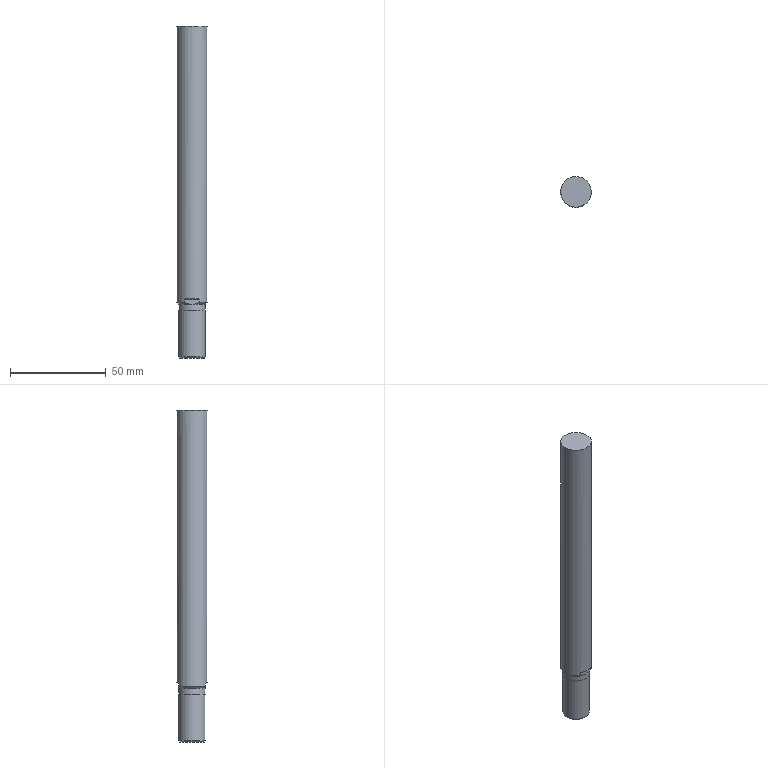Part | STEP file | 冲床-300配套压波_id650_x_t | 1 solid | 14 faces | box 16 x 16 x 173 mm | volume 33408 mm3 | plane 6 | cylinder 5 | cone 3 | commonest cylinder face diameters 1 x2 14 x2 16 x1
STEP:
#1=CARTESIAN_POINT('',(1812.,0.,183.7));
#2=VERTEX_POINT('',#1);
#3=CARTESIAN_POINT('',(1805.,0.,183.7));
#4=DIRECTION('',(0.,0.,1.));
#5=DIRECTION('',(1.,0.,0.));
#6=AXIS2_PLACEMENT_3D('',#3,#4,#5);
#7=CIRCLE('',#6,7.);
#8=EDGE_CURVE('',#2,#2,#7,.T.);
#9=ORIENTED_EDGE('',*,*,#8,.T.);
#10=EDGE_LOOP('',(#9));
#11=FACE_BOUND('',#10,.T.);
#12=CARTESIAN_POINT('',(1798.,0.,208.));
#13=VERTEX_POINT('',#12);
#14=CARTESIAN_POINT('',(1805.,0.,208.));
#15=DIRECTION('',(0.,0.,-1.));
#16=DIRECTION('',(-1.,0.,0.));
#17=AXIS2_PLACEMENT_3D('',#14,#15,#16);
#18=CIRCLE('',#17,7.);
#19=EDGE_CURVE('',#13,#13,#18,.T.);
#20=ORIENTED_EDGE('',*,*,#19,.T.);
#21=EDGE_LOOP('',(#20));
#22=FACE_BOUND('',#21,.T.);
#23=CARTESIAN_POINT('',(1805.,0.,211.));
#24=DIRECTION('',(0.,0.,-1.));
#25=DIRECTION('',(1.,0.,0.));
#26=AXIS2_PLACEMENT_3D('',#23,#24,#25);
#27=CYLINDRICAL_SURFACE('',#26,7.);
#28=ADVANCED_FACE('',(#11,#22),#27,.T.);
#29=CARTESIAN_POINT('',(1801.127,7.,213.3));
#30=VERTEX_POINT('',#29);
#31=CARTESIAN_POINT('',(1801.127,7.,212.));
#32=VERTEX_POINT('',#31);
#33=CARTESIAN_POINT('',(1801.127,7.,213.8));
#34=DIRECTION('',(0.,0.,-1.));
#35=VECTOR('',#34,1.);
#36=LINE('',#33,#35);
#37=EDGE_CURVE('',#30,#32,#36,.T.);
#38=ORIENTED_EDGE('',*,*,#37,.T.);
#39=CARTESIAN_POINT('',(1801.127,-7.,212.));
#40=VERTEX_POINT('',#39);
#41=CARTESIAN_POINT('',(1805.,0.,212.));
#42=DIRECTION('',(0.,0.,1.));
#43=DIRECTION('',(-1.,0.,0.));
#44=AXIS2_PLACEMENT_3D('',#41,#42,#43);
#45=CIRCLE('',#44,8.);
#46=EDGE_CURVE('',#32,#40,#45,.T.);
#47=ORIENTED_EDGE('',*,*,#46,.T.);
#48=CARTESIAN_POINT('',(1801.127,-7.,213.3));
#49=VERTEX_POINT('',#48);
#50=CARTESIAN_POINT('',(1801.127,-7.,213.8));
#51=DIRECTION('',(0.,0.,-1.));
#52=VECTOR('',#51,1.);
#53=LINE('',#50,#52);
#54=EDGE_CURVE('',#49,#40,#53,.T.);
#55=ORIENTED_EDGE('',*,*,#54,.F.);
#56=CARTESIAN_POINT('',(1802.216,-7.5,213.8));
#57=VERTEX_POINT('',#56);
#58=CARTESIAN_POINT('',(1801.127,-7.,213.3));
#59=CARTESIAN_POINT('',(1801.127,-7.,213.329));
#60=CARTESIAN_POINT('',(1801.132,-7.003,213.358));
#61=CARTESIAN_POINT('',(1801.14,-7.007,213.385));
#62=CARTESIAN_POINT('',(1801.151,-7.013,213.419));
#63=CARTESIAN_POINT('',(1801.167,-7.022,213.45));
#64=CARTESIAN_POINT('',(1801.186,-7.032,213.477));
#65=CARTESIAN_POINT('',(1801.216,-7.048,213.519));
#66=CARTESIAN_POINT('',(1801.253,-7.068,213.555));
#67=CARTESIAN_POINT('',(1801.292,-7.089,213.584));
#68=CARTESIAN_POINT('',(1801.365,-7.127,213.64));
#69=CARTESIAN_POINT('',(1801.449,-7.169,213.678));
#70=CARTESIAN_POINT('',(1801.534,-7.21,213.708));
#71=CARTESIAN_POINT('',(1801.718,-7.298,213.77));
#72=CARTESIAN_POINT('',(1801.916,-7.385,213.793));
#73=CARTESIAN_POINT('',(1802.115,-7.462,213.799));
#74=CARTESIAN_POINT('',(1802.148,-7.475,213.8));
#75=CARTESIAN_POINT('',(1802.182,-7.487,213.8));
#76=CARTESIAN_POINT('',(1802.216,-7.5,213.8));
#77=B_SPLINE_CURVE_WITH_KNOTS('',3,(#58,#59,#60,#61,#62,#63,#64,#65,#66,#67,#68,#69,#70,#71,#72,#73,#74,#75,#76),.UNSPECIFIED.,.F.,.F.,(4,3,3,3,3,3,4),(0.,0.06162,0.1366,0.2512,0.4638,0.9227,1.),.UNSPECIFIED.);
#78=EDGE_CURVE('',#49,#57,#77,.T.);
#79=ORIENTED_EDGE('',*,*,#78,.T.);
#80=CARTESIAN_POINT('',(1807.784,-7.5,213.8));
#81=VERTEX_POINT('',#80);
#82=CARTESIAN_POINT('',(1805.,0.,213.8));
#83=DIRECTION('',(0.,0.,-1.));
#84=DIRECTION('',(-1.,0.,0.));
#85=AXIS2_PLACEMENT_3D('',#82,#83,#84);
#86=CIRCLE('',#85,8.);
#87=EDGE_CURVE('',#81,#57,#86,.T.);
#88=ORIENTED_EDGE('',*,*,#87,.F.);
#89=CARTESIAN_POINT('',(1808.873,-7.,213.3));
#90=VERTEX_POINT('',#89);
#91=CARTESIAN_POINT('',(1807.784,-7.5,213.8));
#92=CARTESIAN_POINT('',(1807.985,-7.425,213.8));
#93=CARTESIAN_POINT('',(1808.186,-7.341,213.785));
#94=CARTESIAN_POINT('',(1808.376,-7.253,213.735));
#95=CARTESIAN_POINT('',(1808.44,-7.223,213.718));
#96=CARTESIAN_POINT('',(1808.504,-7.192,213.696));
#97=CARTESIAN_POINT('',(1808.564,-7.162,213.669));
#98=CARTESIAN_POINT('',(1808.642,-7.123,213.633));
#99=CARTESIAN_POINT('',(1808.719,-7.084,213.586));
#100=CARTESIAN_POINT('',(1808.779,-7.051,213.521));
#101=CARTESIAN_POINT('',(1808.801,-7.039,213.496));
#102=CARTESIAN_POINT('',(1808.822,-7.028,213.469));
#103=CARTESIAN_POINT('',(1808.838,-7.019,213.438));
#104=CARTESIAN_POINT('',(1808.854,-7.011,213.407));
#105=CARTESIAN_POINT('',(1808.866,-7.004,213.373));
#106=CARTESIAN_POINT('',(1808.87,-7.001,213.337));
#107=CARTESIAN_POINT('',(1808.872,-7.,213.325));
#108=CARTESIAN_POINT('',(1808.873,-7.,213.312));
#109=CARTESIAN_POINT('',(1808.873,-7.,213.3));
#110=B_SPLINE_CURVE_WITH_KNOTS('',3,(#91,#92,#93,#94,#95,#96,#97,#98,#99,#100,#101,#102,#103,#104,#105,#106,#107,#108,#109),.UNSPECIFIED.,.F.,.F.,(4,3,3,3,3,3,4),(0.,0.4621,0.6184,0.8217,0.8971,0.9738,1.),.UNSPECIFIED.);
#111=EDGE_CURVE('',#81,#90,#110,.T.);
#112=ORIENTED_EDGE('',*,*,#111,.T.);
#113=CARTESIAN_POINT('',(1808.873,-7.,212.));
#114=VERTEX_POINT('',#113);
#115=CARTESIAN_POINT('',(1808.873,-7.,213.8));
#116=DIRECTION('',(0.,0.,1.));
#117=VECTOR('',#116,1.);
#118=LINE('',#115,#117);
#119=EDGE_CURVE('',#114,#90,#118,.T.);
#120=ORIENTED_EDGE('',*,*,#119,.F.);
#121=CARTESIAN_POINT('',(1808.873,7.,212.));
#122=VERTEX_POINT('',#121);
#123=CARTESIAN_POINT('',(1805.,0.,212.));
#124=DIRECTION('',(0.,0.,1.));
#125=DIRECTION('',(-1.,0.,0.));
#126=AXIS2_PLACEMENT_3D('',#123,#124,#125);
#127=CIRCLE('',#126,8.);
#128=EDGE_CURVE('',#114,#122,#127,.T.);
#129=ORIENTED_EDGE('',*,*,#128,.T.);
#130=CARTESIAN_POINT('',(1808.873,7.,213.3));
#131=VERTEX_POINT('',#130);
#132=CARTESIAN_POINT('',(1808.873,7.,213.8));
#133=DIRECTION('',(0.,0.,1.));
#134=VECTOR('',#133,1.);
#135=LINE('',#132,#134);
#136=EDGE_CURVE('',#122,#131,#135,.T.);
#137=ORIENTED_EDGE('',*,*,#136,.T.);
#138=CARTESIAN_POINT('',(1807.784,7.5,213.8));
#139=VERTEX_POINT('',#138);
#140=CARTESIAN_POINT('',(1808.873,7.,213.3));
#141=CARTESIAN_POINT('',(1808.873,7.,213.329));
#142=CARTESIAN_POINT('',(1808.868,7.003,213.358));
#143=CARTESIAN_POINT('',(1808.86,7.007,213.385));
#144=CARTESIAN_POINT('',(1808.849,7.013,213.419));
#145=CARTESIAN_POINT('',(1808.833,7.022,213.45));
#146=CARTESIAN_POINT('',(1808.814,7.032,213.477));
#147=CARTESIAN_POINT('',(1808.784,7.048,213.519));
#148=CARTESIAN_POINT('',(1808.747,7.068,213.555));
#149=CARTESIAN_POINT('',(1808.708,7.089,213.584));
#150=CARTESIAN_POINT('',(1808.635,7.127,213.64));
#151=CARTESIAN_POINT('',(1808.551,7.169,213.678));
#152=CARTESIAN_POINT('',(1808.466,7.21,213.708));
#153=CARTESIAN_POINT('',(1808.282,7.298,213.77));
#154=CARTESIAN_POINT('',(1808.084,7.385,213.793));
#155=CARTESIAN_POINT('',(1807.885,7.462,213.799));
#156=CARTESIAN_POINT('',(1807.852,7.475,213.8));
#157=CARTESIAN_POINT('',(1807.818,7.487,213.8));
#158=CARTESIAN_POINT('',(1807.784,7.5,213.8));
#159=B_SPLINE_CURVE_WITH_KNOTS('',3,(#140,#141,#142,#143,#144,#145,#146,#147,#148,#149,#150,#151,#152,#153,#154,#155,#156,#157,#158),.UNSPECIFIED.,.F.,.F.,(4,3,3,3,3,3,4),(0.,0.06162,0.1366,0.2512,0.4638,0.9227,1.),.UNSPECIFIED.);
#160=EDGE_CURVE('',#131,#139,#159,.T.);
#161=ORIENTED_EDGE('',*,*,#160,.T.);
#162=CARTESIAN_POINT('',(1802.216,7.5,213.8));
#163=VERTEX_POINT('',#162);
#164=CARTESIAN_POINT('',(1805.,0.,213.8));
#165=DIRECTION('',(0.,0.,-1.));
#166=DIRECTION('',(-1.,0.,0.));
#167=AXIS2_PLACEMENT_3D('',#164,#165,#166);
#168=CIRCLE('',#167,8.);
#169=EDGE_CURVE('',#163,#139,#168,.T.);
#170=ORIENTED_EDGE('',*,*,#169,.F.);
#171=CARTESIAN_POINT('',(1802.216,7.5,213.8));
#172=CARTESIAN_POINT('',(1802.015,7.425,213.8));
#173=CARTESIAN_POINT('',(1801.814,7.341,213.785));
#174=CARTESIAN_POINT('',(1801.624,7.253,213.735));
#175=CARTESIAN_POINT('',(1801.56,7.223,213.718));
#176=CARTESIAN_POINT('',(1801.496,7.192,213.696));
#177=CARTESIAN_POINT('',(1801.436,7.162,213.669));
#178=CARTESIAN_POINT('',(1801.358,7.123,213.633));
#179=CARTESIAN_POINT('',(1801.281,7.084,213.586));
#180=CARTESIAN_POINT('',(1801.221,7.051,213.521));
#181=CARTESIAN_POINT('',(1801.199,7.039,213.496));
#182=CARTESIAN_POINT('',(1801.178,7.028,213.469));
#183=CARTESIAN_POINT('',(1801.162,7.019,213.438));
#184=CARTESIAN_POINT('',(1801.146,7.011,213.407));
#185=CARTESIAN_POINT('',(1801.134,7.004,213.373));
#186=CARTESIAN_POINT('',(1801.13,7.001,213.337));
#187=CARTESIAN_POINT('',(1801.128,7.,213.325));
#188=CARTESIAN_POINT('',(1801.127,7.,213.312));
#189=CARTESIAN_POINT('',(1801.127,7.,213.3));
#190=B_SPLINE_CURVE_WITH_KNOTS('',3,(#171,#172,#173,#174,#175,#176,#177,#178,#179,#180,#181,#182,#183,#184,#185,#186,#187,#188,#189),.UNSPECIFIED.,.F.,.F.,(4,3,3,3,3,3,4),(0.,0.4621,0.6184,0.8217,0.8971,0.9738,1.),.UNSPECIFIED.);
#191=EDGE_CURVE('',#163,#30,#190,.T.);
#192=ORIENTED_EDGE('',*,*,#191,.T.);
#193=EDGE_LOOP('',(#38,#47,#55,#79,#88,#112,#120,#129,#137,#161,#170,#192));
#194=FACE_BOUND('',#193,.T.);
#195=CARTESIAN_POINT('',(1805.,8.,356.));
#196=VERTEX_POINT('',#195);
#197=CARTESIAN_POINT('',(1805.,0.,356.));
#198=DIRECTION('',(0.,0.,1.));
#199=DIRECTION('',(0.,1.,0.));
#200=AXIS2_PLACEMENT_3D('',#197,#198,#199);
#201=CIRCLE('',#200,8.);
#202=EDGE_CURVE('',#196,#196,#201,.T.);
#203=ORIENTED_EDGE('',*,*,#202,.F.);
#204=EDGE_LOOP('',(#203));
#205=FACE_BOUND('',#204,.T.);
#206=CARTESIAN_POINT('',(1805.,0.,356.));
#207=DIRECTION('',(0.,0.,-1.));
#208=DIRECTION('',(1.,0.,0.));
#209=AXIS2_PLACEMENT_3D('',#206,#207,#208);
#210=CYLINDRICAL_SURFACE('',#209,8.);
#211=ADVANCED_FACE('',(#194,#205),#210,.T.);
#212=ORIENTED_EDGE('',*,*,#202,.T.);
#213=EDGE_LOOP('',(#212));
#214=FACE_OUTER_BOUND('',#213,.T.);
#215=CARTESIAN_POINT('',(1805.,0.,356.));
#216=DIRECTION('',(0.,0.,1.));
#217=DIRECTION('',(-1.,0.,0.));
#218=AXIS2_PLACEMENT_3D('',#215,#216,#217);
#219=PLANE('',#218);
#220=ADVANCED_FACE('',(#214),#219,.T.);
#221=ORIENTED_EDGE('',*,*,#19,.F.);
#222=EDGE_LOOP('',(#221));
#223=FACE_BOUND('',#222,.T.);
#224=CARTESIAN_POINT('',(1805.,7.,211.));
#225=VERTEX_POINT('',#224);
#226=CARTESIAN_POINT('',(1805.,-7.,211.));
#227=VERTEX_POINT('',#226);
#228=CARTESIAN_POINT('',(1805.,0.,211.));
#229=DIRECTION('',(0.,0.,1.));
#230=DIRECTION('',(0.,1.,0.));
#231=AXIS2_PLACEMENT_3D('',#228,#229,#230);
#232=CIRCLE('',#231,7.);
#233=EDGE_CURVE('',#225,#227,#232,.T.);
#234=ORIENTED_EDGE('',*,*,#233,.F.);
#235=CARTESIAN_POINT('',(1805.,0.,211.));
#236=DIRECTION('',(0.,0.,1.));
#237=DIRECTION('',(0.,1.,0.));
#238=AXIS2_PLACEMENT_3D('',#235,#236,#237);
#239=CIRCLE('',#238,7.);
#240=EDGE_CURVE('',#227,#225,#239,.T.);
#241=ORIENTED_EDGE('',*,*,#240,.F.);
#242=EDGE_LOOP('',(#234,#241));
#243=FACE_BOUND('',#242,.T.);
#244=CARTESIAN_POINT('',(1805.,0.,211.));
#245=DIRECTION('',(0.,0.,-1.));
#246=DIRECTION('',(1.,0.,0.));
#247=AXIS2_PLACEMENT_3D('',#244,#245,#246);
#248=CYLINDRICAL_SURFACE('',#247,7.);
#249=ADVANCED_FACE('',(#223,#243),#248,.T.);
#250=CARTESIAN_POINT('',(1811.3,0.,183.));
#251=VERTEX_POINT('',#250);
#252=CARTESIAN_POINT('',(1805.,0.,183.));
#253=DIRECTION('',(0.,0.,-1.));
#254=DIRECTION('',(1.,0.,0.));
#255=AXIS2_PLACEMENT_3D('',#252,#253,#254);
#256=CIRCLE('',#255,6.3);
#257=EDGE_CURVE('',#251,#251,#256,.T.);
#258=ORIENTED_EDGE('',*,*,#257,.T.);
#259=EDGE_LOOP('',(#258));
#260=FACE_OUTER_BOUND('',#259,.T.);
#261=CARTESIAN_POINT('',(1805.,0.,183.));
#262=DIRECTION('',(0.,0.,1.));
#263=DIRECTION('',(-1.,0.,0.));
#264=AXIS2_PLACEMENT_3D('',#261,#262,#263);
#265=PLANE('',#264);
#266=ADVANCED_FACE('',(#260),#265,.F.);
#267=ORIENTED_EDGE('',*,*,#169,.T.);
#268=CARTESIAN_POINT('',(1805.,7.5,213.8));
#269=DIRECTION('',(-1.,0.,0.));
#270=VECTOR('',#269,1.);
#271=LINE('',#268,#270);
#272=EDGE_CURVE('',#139,#163,#271,.T.);
#273=ORIENTED_EDGE('',*,*,#272,.T.);
#274=EDGE_LOOP('',(#267,#273));
#275=FACE_OUTER_BOUND('',#274,.T.);
#276=CARTESIAN_POINT('',(1805.,7.,213.8));
#277=DIRECTION('',(0.,0.,-1.));
#278=DIRECTION('',(1.,0.,0.));
#279=AXIS2_PLACEMENT_3D('',#276,#277,#278);
#280=PLANE('',#279);
#281=ADVANCED_FACE('',(#275),#280,.T.);
#282=CARTESIAN_POINT('',(1808.873,7.,212.));
#283=CARTESIAN_POINT('',(1807.655,7.,211.41));
#284=CARTESIAN_POINT('',(1806.365,7.,211.));
#285=CARTESIAN_POINT('',(1805.,7.,211.));
#286=B_SPLINE_CURVE_WITH_KNOTS('',3,(#282,#283,#284,#285),.UNSPECIFIED.,.F.,.F.,(4,4),(0.,1.),.UNSPECIFIED.);
#287=EDGE_CURVE('',#122,#225,#286,.T.);
#288=ORIENTED_EDGE('',*,*,#287,.T.);
#289=CARTESIAN_POINT('',(1805.,7.,211.));
#290=CARTESIAN_POINT('',(1803.644,7.,211.));
#291=CARTESIAN_POINT('',(1802.343,7.,211.411));
#292=CARTESIAN_POINT('',(1801.127,7.,212.));
#293=B_SPLINE_CURVE_WITH_KNOTS('',3,(#289,#290,#291,#292),.UNSPECIFIED.,.F.,.F.,(4,4),(0.,1.),.UNSPECIFIED.);
#294=EDGE_CURVE('',#225,#32,#293,.T.);
#295=ORIENTED_EDGE('',*,*,#294,.T.);
#296=ORIENTED_EDGE('',*,*,#37,.F.);
#297=CARTESIAN_POINT('',(1808.873,7.,213.3));
#298=DIRECTION('',(1.,0.,0.));
#299=VECTOR('',#298,1.);
#300=LINE('',#297,#299);
#301=EDGE_CURVE('',#30,#131,#300,.T.);
#302=ORIENTED_EDGE('',*,*,#301,.T.);
#303=ORIENTED_EDGE('',*,*,#136,.F.);
#304=EDGE_LOOP('',(#288,#295,#296,#302,#303));
#305=FACE_OUTER_BOUND('',#304,.T.);
#306=CARTESIAN_POINT('',(1808.873,7.,213.8));
#307=DIRECTION('',(0.,-1.,0.));
#308=DIRECTION('',(-1.,0.,0.));
#309=AXIS2_PLACEMENT_3D('',#306,#307,#308);
#310=PLANE('',#309);
#311=ADVANCED_FACE('',(#305),#310,.F.);
#312=ORIENTED_EDGE('',*,*,#160,.F.);
#313=ORIENTED_EDGE('',*,*,#301,.F.);
#314=ORIENTED_EDGE('',*,*,#191,.F.);
#315=ORIENTED_EDGE('',*,*,#272,.F.);
#316=EDGE_LOOP('',(#312,#313,#314,#315));
#317=FACE_OUTER_BOUND('',#316,.T.);
#318=CARTESIAN_POINT('',(1805.,7.5,213.3));
#319=DIRECTION('',(-1.,0.,0.));
#320=DIRECTION('',(0.,1.,0.));
#321=AXIS2_PLACEMENT_3D('',#318,#319,#320);
#322=CYLINDRICAL_SURFACE('',#321,0.5);
#323=ADVANCED_FACE('',(#317),#322,.F.);
#324=ORIENTED_EDGE('',*,*,#87,.T.);
#325=CARTESIAN_POINT('',(1805.,-7.5,213.8));
#326=DIRECTION('',(1.,0.,0.));
#327=VECTOR('',#326,1.);
#328=LINE('',#325,#327);
#329=EDGE_CURVE('',#57,#81,#328,.T.);
#330=ORIENTED_EDGE('',*,*,#329,.T.);
#331=EDGE_LOOP('',(#324,#330));
#332=FACE_OUTER_BOUND('',#331,.T.);
#333=CARTESIAN_POINT('',(1805.,-7.,213.8));
#334=DIRECTION('',(0.,0.,-1.));
#335=DIRECTION('',(1.,0.,0.));
#336=AXIS2_PLACEMENT_3D('',#333,#334,#335);
#337=PLANE('',#336);
#338=ADVANCED_FACE('',(#332),#337,.T.);
#339=ORIENTED_EDGE('',*,*,#54,.T.);
#340=CARTESIAN_POINT('',(1801.127,-7.,212.));
#341=CARTESIAN_POINT('',(1802.345,-7.,211.41));
#342=CARTESIAN_POINT('',(1803.635,-7.,211.));
#343=CARTESIAN_POINT('',(1805.,-7.,211.));
#344=B_SPLINE_CURVE_WITH_KNOTS('',3,(#340,#341,#342,#343),.UNSPECIFIED.,.F.,.F.,(4,4),(0.,1.),.UNSPECIFIED.);
#345=EDGE_CURVE('',#40,#227,#344,.T.);
#346=ORIENTED_EDGE('',*,*,#345,.T.);
#347=CARTESIAN_POINT('',(1805.,-7.,211.));
#348=CARTESIAN_POINT('',(1806.356,-7.,211.));
#349=CARTESIAN_POINT('',(1807.657,-7.,211.411));
#350=CARTESIAN_POINT('',(1808.873,-7.,212.));
#351=B_SPLINE_CURVE_WITH_KNOTS('',3,(#347,#348,#349,#350),.UNSPECIFIED.,.F.,.F.,(4,4),(0.,1.),.UNSPECIFIED.);
#352=EDGE_CURVE('',#227,#114,#351,.T.);
#353=ORIENTED_EDGE('',*,*,#352,.T.);
#354=ORIENTED_EDGE('',*,*,#119,.T.);
#355=CARTESIAN_POINT('',(1801.127,-7.,213.3));
#356=DIRECTION('',(-1.,0.,0.));
#357=VECTOR('',#356,1.);
#358=LINE('',#355,#357);
#359=EDGE_CURVE('',#90,#49,#358,.T.);
#360=ORIENTED_EDGE('',*,*,#359,.T.);
#361=EDGE_LOOP('',(#339,#346,#353,#354,#360));
#362=FACE_OUTER_BOUND('',#361,.T.);
#363=CARTESIAN_POINT('',(1801.127,-7.,213.8));
#364=DIRECTION('',(0.,1.,0.));
#365=DIRECTION('',(1.,0.,0.));
#366=AXIS2_PLACEMENT_3D('',#363,#364,#365);
#367=PLANE('',#366);
#368=ADVANCED_FACE('',(#362),#367,.F.);
#369=ORIENTED_EDGE('',*,*,#78,.F.);
#370=ORIENTED_EDGE('',*,*,#359,.F.);
#371=ORIENTED_EDGE('',*,*,#111,.F.);
#372=ORIENTED_EDGE('',*,*,#329,.F.);
#373=EDGE_LOOP('',(#369,#370,#371,#372));
#374=FACE_OUTER_BOUND('',#373,.T.);
#375=CARTESIAN_POINT('',(1805.,-7.5,213.3));
#376=DIRECTION('',(1.,0.,0.));
#377=DIRECTION('',(0.,-1.,0.));
#378=AXIS2_PLACEMENT_3D('',#375,#376,#377);
#379=CYLINDRICAL_SURFACE('',#378,0.5);
#380=ADVANCED_FACE('',(#374),#379,.F.);
#381=ORIENTED_EDGE('',*,*,#345,.F.);
#382=ORIENTED_EDGE('',*,*,#46,.F.);
#383=ORIENTED_EDGE('',*,*,#294,.F.);
#384=ORIENTED_EDGE('',*,*,#233,.T.);
#385=EDGE_LOOP('',(#381,#382,#383,#384));
#386=FACE_OUTER_BOUND('',#385,.T.);
#387=CARTESIAN_POINT('',(1805.,0.,211.));
#388=DIRECTION('',(0.,0.,1.));
#389=DIRECTION('',(-1.,0.,0.));
#390=AXIS2_PLACEMENT_3D('',#387,#388,#389);
#391=CONICAL_SURFACE('',#390,7.,45.);
#392=ADVANCED_FACE('',(#386),#391,.T.);
#393=ORIENTED_EDGE('',*,*,#287,.F.);
#394=ORIENTED_EDGE('',*,*,#128,.F.);
#395=ORIENTED_EDGE('',*,*,#352,.F.);
#396=ORIENTED_EDGE('',*,*,#240,.T.);
#397=EDGE_LOOP('',(#393,#394,#395,#396));
#398=FACE_OUTER_BOUND('',#397,.T.);
#399=CARTESIAN_POINT('',(1805.,0.,211.));
#400=DIRECTION('',(0.,0.,1.));
#401=DIRECTION('',(-1.,0.,0.));
#402=AXIS2_PLACEMENT_3D('',#399,#400,#401);
#403=CONICAL_SURFACE('',#402,7.,45.);
#404=ADVANCED_FACE('',(#398),#403,.T.);
#405=ORIENTED_EDGE('',*,*,#257,.F.);
#406=EDGE_LOOP('',(#405));
#407=FACE_BOUND('',#406,.T.);
#408=ORIENTED_EDGE('',*,*,#8,.F.);
#409=EDGE_LOOP('',(#408));
#410=FACE_BOUND('',#409,.T.);
#411=CARTESIAN_POINT('',(1805.,0.,183.7));
#412=DIRECTION('',(0.,0.,1.));
#413=DIRECTION('',(-1.,0.,0.));
#414=AXIS2_PLACEMENT_3D('',#411,#412,#413);
#415=CONICAL_SURFACE('',#414,7.,45.);
#416=ADVANCED_FACE('',(#407,#410),#415,.T.);
#417=CLOSED_SHELL('',(#28,#211,#220,#249,#266,#281,#311,#323,#338,#368,#380,#392,#404,#416));
#418=MANIFOLD_SOLID_BREP('',#417);
#419=(LENGTH_UNIT()NAMED_UNIT(*)SI_UNIT(.MILLI.,.METRE.));
#420=UNCERTAINTY_MEASURE_WITH_UNIT(LENGTH_MEASURE(0.0508),#419,'','');
#421=(NAMED_UNIT(*)PLANE_ANGLE_UNIT()SI_UNIT($,.RADIAN.));
#422=PLANE_ANGLE_MEASURE_WITH_UNIT(PLANE_ANGLE_MEASURE(0.01745),#421);
#423=DIMENSIONAL_EXPONENTS(0.,0.,0.,0.,0.,0.,0.);
#424=(CONVERSION_BASED_UNIT('DEGREE',#422)NAMED_UNIT(#423)PLANE_ANGLE_UNIT());
#425=(NAMED_UNIT(*)SI_UNIT($,.STERADIAN.)SOLID_ANGLE_UNIT());
#426=(GEOMETRIC_REPRESENTATION_CONTEXT(3)GLOBAL_UNCERTAINTY_ASSIGNED_CONTEXT((#420))GLOBAL_UNIT_ASSIGNED_CONTEXT((#419,#424,#425))REPRESENTATION_CONTEXT('',''));
#427=ADVANCED_BREP_SHAPE_REPRESENTATION('',(#418),#426);